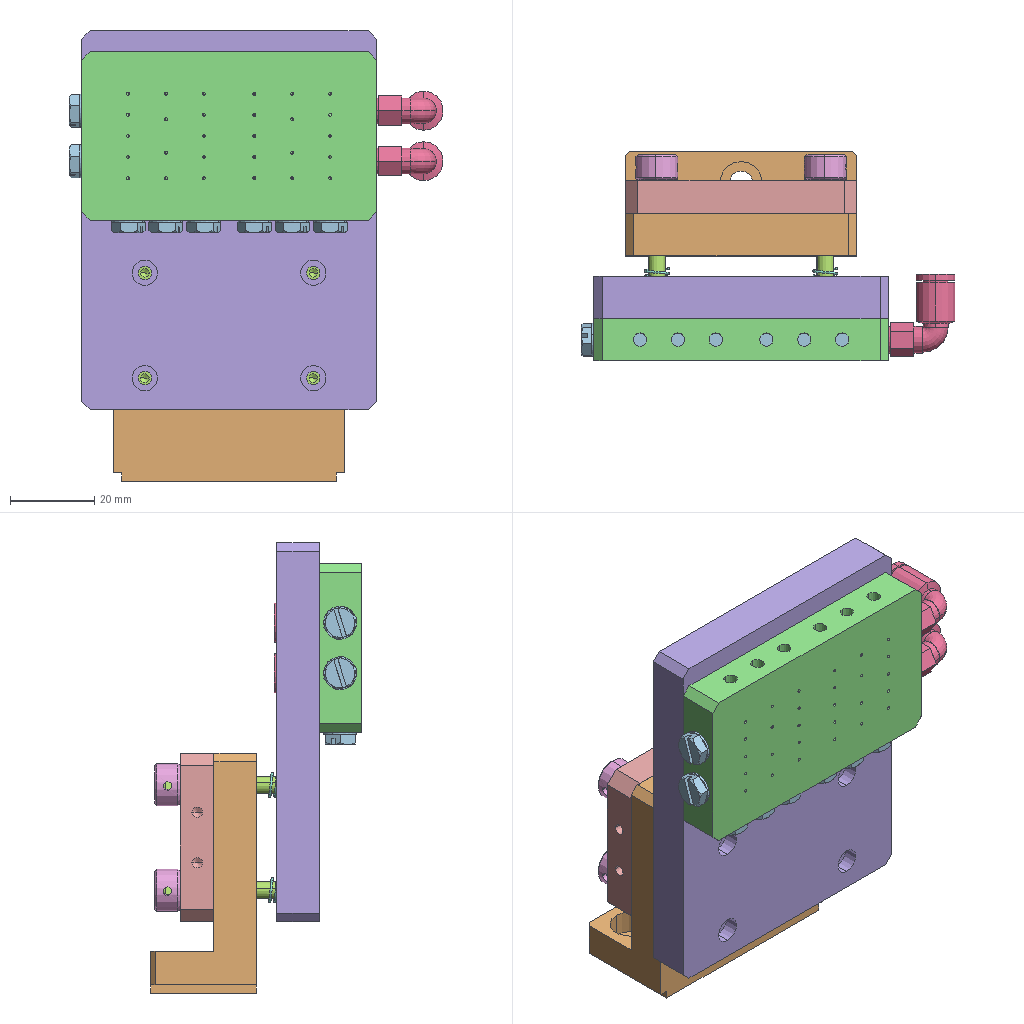Assembly | SolidWorks | 11 different items | 34 placed | box 89 x 50 x 107 mm
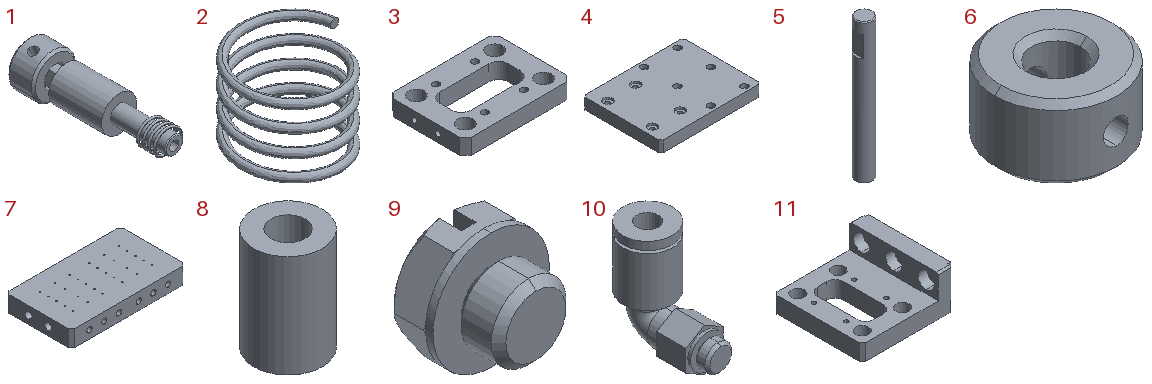Parts list (item | name | quantity | parent item | size | volume | features):
1 | (subassembly) | x4 | - | 10 x 33 x 10 mm | 1213 mm3 | features CompositeCurve 1
2 | - | x4 | in 1 | 6 x 6 x 5.5 mm | 13.577 mm3 | features Helix 1, Sweep 1
3 | - | x1 | - | 55 x 40 x 8 mm | 11071 mm3 | features HoleWzd 4, Chamfer 1, Extrusion 1, Fillet 1, ICE 1
4 | - | x1 | - | 90 x 70 x 10 mm | 61013 mm3 | features HoleWzd 2, ICE 2, Chamfer 1, Extrusion 1
5 | - | x4 | in 1 | 4 x 4 x 33 mm | 382.151 mm3 | features BaseBody 1, Chamfer 1
6 | - | x4 | in 1 | 10 x 10 x 6 mm | 364.767 mm3 | features BaseBody 1, Chamfer 1
7 | - | x1 | - | 70 x 40 x 10 mm | 24196 mm3 | features HoleWzd 8, LPattern 2, Chamfer 1, Extrusion 1
8 | - | x4 | in 1 | 8 x 8 x 12 mm | 452.389 mm3 | features BaseBody 1
9 | - | x8 | - | 8.083 x 6 x 7.8 mm | 174.211 mm3 | features BaseBody 1
10 | - | x2 | - | 9.3 x 18.35 x 19.641 mm | 1123 mm3 | features BaseBody 1
11 | - | x1 | - | 57 x 55 x 25 mm | 30548 mm3 | features HoleWzd 3, ICE 3, Chamfer 2, Extrusion 1, Fillet 1
Mates (type | each side: item.copy, entity, surface, feature):
In the top assembly
Coincident | 5.1 face plane 输入1 | 4.1 face plane Cut-Extrude 2
Concentric | 5.1 face cylinder 输入1 | 4.1 face cylinder Cut-Extrude 2
Parallel | 1.1 plane | 4.1 face plane Boss-Extrude 1
Concentric | 11.1 face cylinder 打Hole尺寸(%根据)内六角圆柱头Screw的类型1 | 4.1 face cylinder Cut-Extrude 2 | 2 times
Coincident | 8.1 face plane 输入1 | 11.1 face plane 打Hole尺寸(%根据)内六角圆柱头Screw的类型1
Coincident | 3.1 face plane Boss-Extrude 1 | 11.1 face plane Boss-Extrude 1 | 2 times
Concentric | 3.1 face cylinder M8x1.0 Tapped Hole 1 | 8.1 face cylinder 输入1
Coincident | 4.1 face plane Cut-Extrude 2 | 5.2 face plane 输入1
Concentric | 4.1 face cylinder Cut-Extrude 1 | 8.2 face cylinder 输入1
Coincident | 4.1 face plane Cut-Extrude 2 | 5.3 face plane 输入1
Concentric | 4.1 face cylinder Cut-Extrude 2 | 5.3 face cylinder 输入1
Coincident | 4.1 face plane Cut-Extrude 2 | 5.4 face plane 输入1
Concentric | 4.1 face cylinder Cut-Extrude 2 | 5.4 face cylinder 输入1
Coincident | 8.1 face plane 输入1 | 8.2 face plane 输入1
Coincident | 8.1 face plane 输入1 | 8.3 face plane 输入1
Coincident | 8.1 face plane 输入1 | 8.4 face plane 输入1
Coincident | 4.1 plane | assembly plane | 3 times
Concentric | 7.1 face cylinder M5 Tapped Hole 4 | 9.1 face cylinder 输入1
Coincident | 7.1 face plane Boss-Extrude 1 | 9.1 face plane 输入1
Parallel | 7.1 face plane Boss-Extrude 1 | 9.1 face plane 输入1
Concentric | 7.1 face cylinder M5 Tapped Hole 4 | 9.2 face cylinder 输入1
Coincident | 7.1 face plane Boss-Extrude 1 | 9.2 face plane 输入1
Coincident | 4.1 face plane Boss-Extrude 1 | 7.1 face plane Boss-Extrude 1
Concentric | 4.1 face cylinder 打Hole尺寸(%根据)内六角圆柱头Screw的类型1 | 7.1 face cylinder M3 Tapped Hole 2 | 2 times
Concentric | 7.1 face cylinder M5 Tapped Hole 2 | 10.1 face cylinder 输入1
Coincident | 7.1 face plane Boss-Extrude 1 | 10.1 face plane 输入1
Parallel | 7.1 face plane Boss-Extrude 1 | 10.1 face plane 输入1
Coincident | 7.1 face plane Boss-Extrude 1 | 10.2 face plane 输入1
Concentric | 7.1 face cylinder M5 Tapped Hole 2 | 10.2 face cylinder 输入1
Parallel | 7.1 face plane Boss-Extrude 1 | 10.2 face plane 输入1
Concentric | 7.1 face cylinder M5 Tapped Hole 1 | 9.3 face cylinder 输入1
Coincident | 7.1 face plane Boss-Extrude 1 | 9.3 face plane 输入1
Concentric | 7.1 face cylinder M5 Tapped Hole 1 | 9.4 face cylinder 输入1
Coincident | 7.1 face plane Boss-Extrude 1 | 9.4 face plane 输入1
In subassembly 1
Concentric | 5.5 face cylinder 输入1 | 8.5 face cylinder 输入1
Coincident | 5.5 face plane 输入1 | 6.1 face plane 输入1
Concentric | 5.5 face cylinder 输入1 | 6.1 face cylinder 输入1
LimitDistanceDim | 8.5 face plane 输入1 | 6.1 face plane 输入1
Coincident | 8.5 plane | 1.2 plane | 3 times
Concentric | 5.5 face cylinder 输入1 | 2.1 select_type:24
DistanceDim | 2.1 plane | 5.5 face plane 输入1